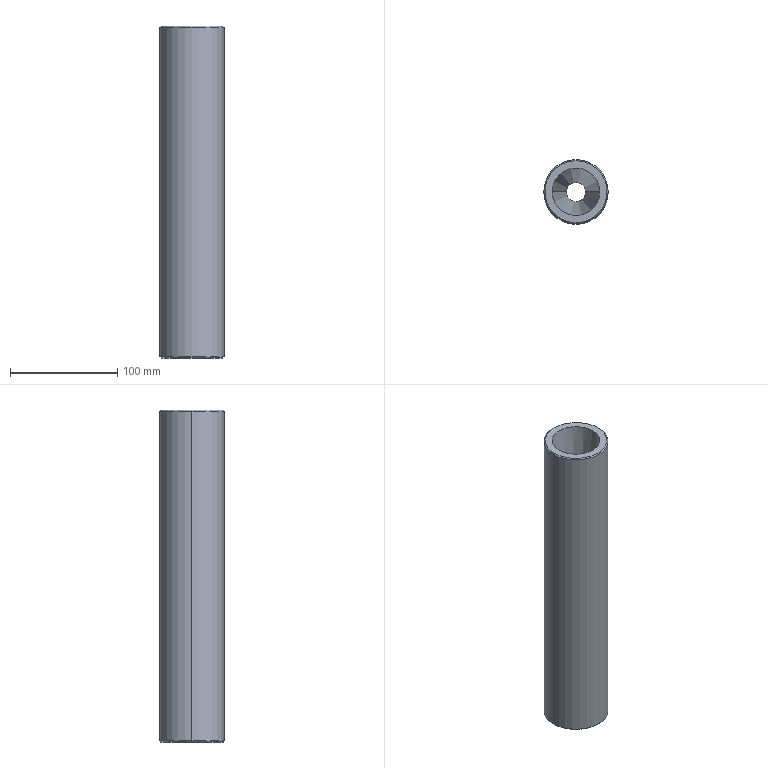Part | STEP file | Tailstock Sleeve | 1 solid | 17 faces | box 60 x 60 x 310 mm | volume 687459 mm3 | cone 8 | cylinder 6 | plane 3 | commonest cylinder face diameters 18 x2 33.5 x2 60 x2
STEP:
#1=CARTESIAN_POINT('',(0.,30.,-154.));
#2=VERTEX_POINT('',#1);
#3=CARTESIAN_POINT('',(-30.,0.,-154.));
#4=VERTEX_POINT('',#3);
#5=CARTESIAN_POINT('',(0.,0.,-154.));
#6=DIRECTION('',(0.,0.,1.));
#7=DIRECTION('',(1.,0.,0.));
#8=AXIS2_PLACEMENT_3D('',#5,#6,#7);
#9=CIRCLE('',#8,30.);
#10=EDGE_CURVE('',#2,#4,#9,.T.);
#11=ORIENTED_EDGE('',*,*,#10,.T.);
#12=CARTESIAN_POINT('',(-30.,0.,154.));
#13=VERTEX_POINT('',#12);
#14=CARTESIAN_POINT('',(-30.,0.,0.));
#15=DIRECTION('',(0.,0.,1.));
#16=VECTOR('',#15,1000.);
#17=LINE('',#14,#16);
#18=EDGE_CURVE('',#4,#13,#17,.T.);
#19=ORIENTED_EDGE('',*,*,#18,.T.);
#20=CARTESIAN_POINT('',(0.,30.,154.));
#21=VERTEX_POINT('',#20);
#22=CARTESIAN_POINT('',(0.,0.,154.));
#23=DIRECTION('',(0.,0.,-1.));
#24=DIRECTION('',(1.,0.,0.));
#25=AXIS2_PLACEMENT_3D('',#22,#23,#24);
#26=CIRCLE('',#25,30.);
#27=EDGE_CURVE('',#13,#21,#26,.T.);
#28=ORIENTED_EDGE('',*,*,#27,.T.);
#29=CARTESIAN_POINT('',(30.,0.,154.));
#30=VERTEX_POINT('',#29);
#31=CARTESIAN_POINT('',(0.,0.,154.));
#32=DIRECTION('',(0.,0.,-1.));
#33=DIRECTION('',(1.,0.,0.));
#34=AXIS2_PLACEMENT_3D('',#31,#32,#33);
#35=CIRCLE('',#34,30.);
#36=EDGE_CURVE('',#21,#30,#35,.T.);
#37=ORIENTED_EDGE('',*,*,#36,.T.);
#38=CARTESIAN_POINT('',(30.,0.,-154.));
#39=VERTEX_POINT('',#38);
#40=CARTESIAN_POINT('',(30.,0.,0.));
#41=DIRECTION('',(0.,0.,1.));
#42=VECTOR('',#41,1000.);
#43=LINE('',#40,#42);
#44=EDGE_CURVE('',#39,#30,#43,.T.);
#45=ORIENTED_EDGE('',*,*,#44,.F.);
#46=CARTESIAN_POINT('',(0.,0.,-154.));
#47=DIRECTION('',(0.,0.,1.));
#48=DIRECTION('',(1.,0.,0.));
#49=AXIS2_PLACEMENT_3D('',#46,#47,#48);
#50=CIRCLE('',#49,30.);
#51=EDGE_CURVE('',#39,#2,#50,.T.);
#52=ORIENTED_EDGE('',*,*,#51,.T.);
#53=EDGE_LOOP('',(#11,#19,#28,#37,#45,#52));
#54=FACE_OUTER_BOUND('',#53,.T.);
#55=CARTESIAN_POINT('',(0.,0.,0.));
#56=DIRECTION('',(0.,0.,1.));
#57=DIRECTION('',(1.,0.,0.));
#58=AXIS2_PLACEMENT_3D('',#55,#56,#57);
#59=CYLINDRICAL_SURFACE('',#58,30.);
#60=ADVANCED_FACE('',(#54),#59,.T.);
#61=CARTESIAN_POINT('',(0.,29.,155.));
#62=VERTEX_POINT('',#61);
#63=CARTESIAN_POINT('',(0.,-29.,155.));
#64=VERTEX_POINT('',#63);
#65=CARTESIAN_POINT('',(0.,0.,155.));
#66=DIRECTION('',(0.,0.,-1.));
#67=DIRECTION('',(0.,1.,0.));
#68=AXIS2_PLACEMENT_3D('',#65,#66,#67);
#69=CIRCLE('',#68,29.);
#70=EDGE_CURVE('',#62,#64,#69,.T.);
#71=ORIENTED_EDGE('',*,*,#70,.T.);
#72=CARTESIAN_POINT('',(0.,-30.,154.));
#73=VERTEX_POINT('',#72);
#74=CARTESIAN_POINT('',(0.,-30.,154.));
#75=DIRECTION('',(0.,-0.7071,-0.7071));
#76=VECTOR('',#75,1000.);
#77=LINE('',#74,#76);
#78=EDGE_CURVE('',#64,#73,#77,.T.);
#79=ORIENTED_EDGE('',*,*,#78,.T.);
#80=CARTESIAN_POINT('',(0.,0.,154.));
#81=DIRECTION('',(0.,0.,-1.));
#82=DIRECTION('',(1.,0.,0.));
#83=AXIS2_PLACEMENT_3D('',#80,#81,#82);
#84=CIRCLE('',#83,30.);
#85=EDGE_CURVE('',#30,#73,#84,.T.);
#86=ORIENTED_EDGE('',*,*,#85,.F.);
#87=ORIENTED_EDGE('',*,*,#36,.F.);
#88=CARTESIAN_POINT('',(0.,30.,154.));
#89=DIRECTION('',(0.,0.7071,-0.7071));
#90=VECTOR('',#89,1000.);
#91=LINE('',#88,#90);
#92=EDGE_CURVE('',#62,#21,#91,.T.);
#93=ORIENTED_EDGE('',*,*,#92,.F.);
#94=EDGE_LOOP('',(#71,#79,#86,#87,#93));
#95=FACE_OUTER_BOUND('',#94,.T.);
#96=CARTESIAN_POINT('',(0.,0.,154.));
#97=DIRECTION('',(0.,0.,-1.));
#98=DIRECTION('',(0.,1.,0.));
#99=AXIS2_PLACEMENT_3D('',#96,#97,#98);
#100=CONICAL_SURFACE('',#99,30.,0.7854);
#101=ADVANCED_FACE('',(#95),#100,.T.);
#102=CARTESIAN_POINT('',(0.,-29.,-155.));
#103=VERTEX_POINT('',#102);
#104=CARTESIAN_POINT('',(0.,29.,-155.));
#105=VERTEX_POINT('',#104);
#106=CARTESIAN_POINT('',(0.,0.,-155.));
#107=DIRECTION('',(0.,0.,1.));
#108=DIRECTION('',(0.,-1.,0.));
#109=AXIS2_PLACEMENT_3D('',#106,#107,#108);
#110=CIRCLE('',#109,29.);
#111=EDGE_CURVE('',#103,#105,#110,.T.);
#112=ORIENTED_EDGE('',*,*,#111,.T.);
#113=CARTESIAN_POINT('',(0.,30.,-154.));
#114=DIRECTION('',(0.,0.7071,0.7071));
#115=VECTOR('',#114,1000.);
#116=LINE('',#113,#115);
#117=EDGE_CURVE('',#105,#2,#116,.T.);
#118=ORIENTED_EDGE('',*,*,#117,.T.);
#119=ORIENTED_EDGE('',*,*,#51,.F.);
#120=CARTESIAN_POINT('',(0.,-30.,-154.));
#121=VERTEX_POINT('',#120);
#122=CARTESIAN_POINT('',(0.,0.,-154.));
#123=DIRECTION('',(0.,0.,1.));
#124=DIRECTION('',(1.,0.,0.));
#125=AXIS2_PLACEMENT_3D('',#122,#123,#124);
#126=CIRCLE('',#125,30.);
#127=EDGE_CURVE('',#121,#39,#126,.T.);
#128=ORIENTED_EDGE('',*,*,#127,.F.);
#129=CARTESIAN_POINT('',(0.,-30.,-154.));
#130=DIRECTION('',(0.,-0.7071,0.7071));
#131=VECTOR('',#130,1000.);
#132=LINE('',#129,#131);
#133=EDGE_CURVE('',#103,#121,#132,.T.);
#134=ORIENTED_EDGE('',*,*,#133,.F.);
#135=EDGE_LOOP('',(#112,#118,#119,#128,#134));
#136=FACE_OUTER_BOUND('',#135,.T.);
#137=CARTESIAN_POINT('',(0.,0.,-154.));
#138=DIRECTION('',(0.,0.,1.));
#139=DIRECTION('',(0.,-1.,0.));
#140=AXIS2_PLACEMENT_3D('',#137,#138,#139);
#141=CONICAL_SURFACE('',#140,30.,0.7854);
#142=ADVANCED_FACE('',(#136),#141,.T.);
#143=CARTESIAN_POINT('',(-9.,0.,13.595));
#144=VERTEX_POINT('',#143);
#145=CARTESIAN_POINT('',(9.,0.,13.595));
#146=VERTEX_POINT('',#145);
#147=CARTESIAN_POINT('',(0.,0.,13.595));
#148=DIRECTION('',(0.,0.,1.));
#149=DIRECTION('',(1.,0.,0.));
#150=AXIS2_PLACEMENT_3D('',#147,#148,#149);
#151=CIRCLE('',#150,9.);
#152=EDGE_CURVE('',#144,#146,#151,.T.);
#153=ORIENTED_EDGE('',*,*,#152,.F.);
#154=CARTESIAN_POINT('',(-22.2,0.,155.));
#155=VERTEX_POINT('',#154);
#156=CARTESIAN_POINT('',(-22.2,0.,155.));
#157=DIRECTION('',(-0.09294,0.,0.9957));
#158=VECTOR('',#157,1000.);
#159=LINE('',#156,#158);
#160=EDGE_CURVE('',#144,#155,#159,.T.);
#161=ORIENTED_EDGE('',*,*,#160,.T.);
#162=CARTESIAN_POINT('',(22.2,0.,155.));
#163=VERTEX_POINT('',#162);
#164=CARTESIAN_POINT('',(0.,0.,155.));
#165=DIRECTION('',(0.,0.,1.));
#166=DIRECTION('',(1.,0.,0.));
#167=AXIS2_PLACEMENT_3D('',#164,#165,#166);
#168=CIRCLE('',#167,22.2);
#169=EDGE_CURVE('',#155,#163,#168,.T.);
#170=ORIENTED_EDGE('',*,*,#169,.T.);
#171=CARTESIAN_POINT('',(22.2,0.,155.));
#172=DIRECTION('',(0.09294,0.,0.9957));
#173=VECTOR('',#172,1000.);
#174=LINE('',#171,#173);
#175=EDGE_CURVE('',#146,#163,#174,.T.);
#176=ORIENTED_EDGE('',*,*,#175,.F.);
#177=EDGE_LOOP('',(#153,#161,#170,#176));
#178=FACE_OUTER_BOUND('',#177,.T.);
#179=CARTESIAN_POINT('',(0.,0.,155.));
#180=DIRECTION('',(0.,0.,1.));
#181=DIRECTION('',(1.,0.,0.));
#182=AXIS2_PLACEMENT_3D('',#179,#180,#181);
#183=CONICAL_SURFACE('',#182,22.2,0.09308);
#184=ADVANCED_FACE('',(#178),#183,.F.);
#185=CARTESIAN_POINT('',(16.75,0.,-154.));
#186=VERTEX_POINT('',#185);
#187=CARTESIAN_POINT('',(-16.75,0.,-154.));
#188=VERTEX_POINT('',#187);
#189=CARTESIAN_POINT('',(0.,0.,-154.));
#190=DIRECTION('',(0.,0.,-1.));
#191=DIRECTION('',(-1.,0.,0.));
#192=AXIS2_PLACEMENT_3D('',#189,#190,#191);
#193=CIRCLE('',#192,16.75);
#194=EDGE_CURVE('',#186,#188,#193,.T.);
#195=ORIENTED_EDGE('',*,*,#194,.F.);
#196=CARTESIAN_POINT('',(17.75,0.,-155.));
#197=VERTEX_POINT('',#196);
#198=CARTESIAN_POINT('',(17.75,0.,-155.));
#199=DIRECTION('',(0.7071,0.,-0.7071));
#200=VECTOR('',#199,1000.);
#201=LINE('',#198,#200);
#202=EDGE_CURVE('',#186,#197,#201,.T.);
#203=ORIENTED_EDGE('',*,*,#202,.T.);
#204=CARTESIAN_POINT('',(-17.75,0.,-155.));
#205=VERTEX_POINT('',#204);
#206=CARTESIAN_POINT('',(0.,0.,-155.));
#207=DIRECTION('',(0.,0.,-1.));
#208=DIRECTION('',(-1.,0.,0.));
#209=AXIS2_PLACEMENT_3D('',#206,#207,#208);
#210=CIRCLE('',#209,17.75);
#211=EDGE_CURVE('',#197,#205,#210,.T.);
#212=ORIENTED_EDGE('',*,*,#211,.T.);
#213=CARTESIAN_POINT('',(-17.75,0.,-155.));
#214=DIRECTION('',(-0.7071,0.,-0.7071));
#215=VECTOR('',#214,1000.);
#216=LINE('',#213,#215);
#217=EDGE_CURVE('',#188,#205,#216,.T.);
#218=ORIENTED_EDGE('',*,*,#217,.F.);
#219=EDGE_LOOP('',(#195,#203,#212,#218));
#220=FACE_OUTER_BOUND('',#219,.T.);
#221=CARTESIAN_POINT('',(0.,0.,-155.));
#222=DIRECTION('',(0.,0.,-1.));
#223=DIRECTION('',(-1.,0.,0.));
#224=AXIS2_PLACEMENT_3D('',#221,#222,#223);
#225=CONICAL_SURFACE('',#224,17.75,0.7854);
#226=ADVANCED_FACE('',(#220),#225,.F.);
#227=CARTESIAN_POINT('',(-9.,0.,-105.));
#228=VERTEX_POINT('',#227);
#229=CARTESIAN_POINT('',(9.,0.,-105.));
#230=VERTEX_POINT('',#229);
#231=CARTESIAN_POINT('',(0.,0.,-105.));
#232=DIRECTION('',(0.,0.,1.));
#233=DIRECTION('',(1.,0.,0.));
#234=AXIS2_PLACEMENT_3D('',#231,#232,#233);
#235=CIRCLE('',#234,9.);
#236=EDGE_CURVE('',#228,#230,#235,.T.);
#237=ORIENTED_EDGE('',*,*,#236,.F.);
#238=CARTESIAN_POINT('',(-9.,0.,0.));
#239=DIRECTION('',(0.,0.,1.));
#240=VECTOR('',#239,1000.);
#241=LINE('',#238,#240);
#242=EDGE_CURVE('',#228,#144,#241,.T.);
#243=ORIENTED_EDGE('',*,*,#242,.T.);
#244=ORIENTED_EDGE('',*,*,#152,.T.);
#245=CARTESIAN_POINT('',(9.,0.,0.));
#246=DIRECTION('',(0.,0.,1.));
#247=VECTOR('',#246,1000.);
#248=LINE('',#245,#247);
#249=EDGE_CURVE('',#230,#146,#248,.T.);
#250=ORIENTED_EDGE('',*,*,#249,.F.);
#251=EDGE_LOOP('',(#237,#243,#244,#250));
#252=FACE_OUTER_BOUND('',#251,.T.);
#253=CARTESIAN_POINT('',(0.,0.,0.));
#254=DIRECTION('',(0.,0.,1.));
#255=DIRECTION('',(1.,0.,0.));
#256=AXIS2_PLACEMENT_3D('',#253,#254,#255);
#257=CYLINDRICAL_SURFACE('',#256,9.);
#258=ADVANCED_FACE('',(#252),#257,.F.);
#259=CARTESIAN_POINT('',(16.75,0.,-105.));
#260=VERTEX_POINT('',#259);
#261=CARTESIAN_POINT('',(-16.75,0.,-105.));
#262=VERTEX_POINT('',#261);
#263=CARTESIAN_POINT('',(0.,0.,-105.));
#264=DIRECTION('',(0.,0.,-1.));
#265=DIRECTION('',(-1.,0.,0.));
#266=AXIS2_PLACEMENT_3D('',#263,#264,#265);
#267=CIRCLE('',#266,16.75);
#268=EDGE_CURVE('',#260,#262,#267,.T.);
#269=ORIENTED_EDGE('',*,*,#268,.F.);
#270=CARTESIAN_POINT('',(16.75,0.,-105.));
#271=DIRECTION('',(0.,0.,-1.));
#272=VECTOR('',#271,1000.);
#273=LINE('',#270,#272);
#274=EDGE_CURVE('',#260,#186,#273,.T.);
#275=ORIENTED_EDGE('',*,*,#274,.T.);
#276=ORIENTED_EDGE('',*,*,#194,.T.);
#277=CARTESIAN_POINT('',(-16.75,0.,-105.));
#278=DIRECTION('',(0.,0.,-1.));
#279=VECTOR('',#278,1000.);
#280=LINE('',#277,#279);
#281=EDGE_CURVE('',#262,#188,#280,.T.);
#282=ORIENTED_EDGE('',*,*,#281,.F.);
#283=EDGE_LOOP('',(#269,#275,#276,#282));
#284=FACE_OUTER_BOUND('',#283,.T.);
#285=CARTESIAN_POINT('',(0.,0.,-105.));
#286=DIRECTION('',(0.,0.,-1.));
#287=DIRECTION('',(-1.,0.,0.));
#288=AXIS2_PLACEMENT_3D('',#285,#286,#287);
#289=CYLINDRICAL_SURFACE('',#288,16.75);
#290=ADVANCED_FACE('',(#284),#289,.F.);
#291=ORIENTED_EDGE('',*,*,#18,.F.);
#292=CARTESIAN_POINT('',(0.,0.,-154.));
#293=DIRECTION('',(0.,0.,1.));
#294=DIRECTION('',(1.,0.,0.));
#295=AXIS2_PLACEMENT_3D('',#292,#293,#294);
#296=CIRCLE('',#295,30.);
#297=EDGE_CURVE('',#4,#121,#296,.T.);
#298=ORIENTED_EDGE('',*,*,#297,.T.);
#299=ORIENTED_EDGE('',*,*,#127,.T.);
#300=ORIENTED_EDGE('',*,*,#44,.T.);
#301=ORIENTED_EDGE('',*,*,#85,.T.);
#302=CARTESIAN_POINT('',(0.,0.,154.));
#303=DIRECTION('',(0.,0.,-1.));
#304=DIRECTION('',(1.,0.,0.));
#305=AXIS2_PLACEMENT_3D('',#302,#303,#304);
#306=CIRCLE('',#305,30.);
#307=EDGE_CURVE('',#73,#13,#306,.T.);
#308=ORIENTED_EDGE('',*,*,#307,.T.);
#309=EDGE_LOOP('',(#291,#298,#299,#300,#301,#308));
#310=FACE_OUTER_BOUND('',#309,.T.);
#311=CARTESIAN_POINT('',(0.,0.,0.));
#312=DIRECTION('',(0.,0.,1.));
#313=DIRECTION('',(1.,0.,0.));
#314=AXIS2_PLACEMENT_3D('',#311,#312,#313);
#315=CYLINDRICAL_SURFACE('',#314,30.);
#316=ADVANCED_FACE('',(#310),#315,.T.);
#317=ORIENTED_EDGE('',*,*,#78,.F.);
#318=CARTESIAN_POINT('',(0.,0.,155.));
#319=DIRECTION('',(0.,0.,-1.));
#320=DIRECTION('',(0.,1.,0.));
#321=AXIS2_PLACEMENT_3D('',#318,#319,#320);
#322=CIRCLE('',#321,29.);
#323=EDGE_CURVE('',#64,#62,#322,.T.);
#324=ORIENTED_EDGE('',*,*,#323,.T.);
#325=ORIENTED_EDGE('',*,*,#92,.T.);
#326=ORIENTED_EDGE('',*,*,#27,.F.);
#327=ORIENTED_EDGE('',*,*,#307,.F.);
#328=EDGE_LOOP('',(#317,#324,#325,#326,#327));
#329=FACE_OUTER_BOUND('',#328,.T.);
#330=CARTESIAN_POINT('',(0.,0.,154.));
#331=DIRECTION('',(0.,0.,-1.));
#332=DIRECTION('',(0.,1.,0.));
#333=AXIS2_PLACEMENT_3D('',#330,#331,#332);
#334=CONICAL_SURFACE('',#333,30.,0.7854);
#335=ADVANCED_FACE('',(#329),#334,.T.);
#336=ORIENTED_EDGE('',*,*,#117,.F.);
#337=CARTESIAN_POINT('',(0.,0.,-155.));
#338=DIRECTION('',(0.,0.,1.));
#339=DIRECTION('',(0.,-1.,0.));
#340=AXIS2_PLACEMENT_3D('',#337,#338,#339);
#341=CIRCLE('',#340,29.);
#342=EDGE_CURVE('',#105,#103,#341,.T.);
#343=ORIENTED_EDGE('',*,*,#342,.T.);
#344=ORIENTED_EDGE('',*,*,#133,.T.);
#345=ORIENTED_EDGE('',*,*,#297,.F.);
#346=ORIENTED_EDGE('',*,*,#10,.F.);
#347=EDGE_LOOP('',(#336,#343,#344,#345,#346));
#348=FACE_OUTER_BOUND('',#347,.T.);
#349=CARTESIAN_POINT('',(0.,0.,-154.));
#350=DIRECTION('',(0.,0.,1.));
#351=DIRECTION('',(0.,-1.,0.));
#352=AXIS2_PLACEMENT_3D('',#349,#350,#351);
#353=CONICAL_SURFACE('',#352,30.,0.7854);
#354=ADVANCED_FACE('',(#348),#353,.T.);
#355=CARTESIAN_POINT('',(0.,0.,155.));
#356=DIRECTION('',(0.,0.,1.));
#357=DIRECTION('',(1.,0.,0.));
#358=AXIS2_PLACEMENT_3D('',#355,#356,#357);
#359=CIRCLE('',#358,22.2);
#360=EDGE_CURVE('',#163,#155,#359,.T.);
#361=ORIENTED_EDGE('',*,*,#360,.F.);
#362=ORIENTED_EDGE('',*,*,#169,.F.);
#363=EDGE_LOOP('',(#361,#362));
#364=FACE_BOUND('',#363,.T.);
#365=ORIENTED_EDGE('',*,*,#70,.F.);
#366=ORIENTED_EDGE('',*,*,#323,.F.);
#367=EDGE_LOOP('',(#365,#366));
#368=FACE_OUTER_BOUND('',#367,.T.);
#369=CARTESIAN_POINT('',(0.,30.,155.));
#370=DIRECTION('',(0.,0.,-1.));
#371=DIRECTION('',(-1.,0.,0.));
#372=AXIS2_PLACEMENT_3D('',#369,#370,#371);
#373=PLANE('',#372);
#374=ADVANCED_FACE('',(#364,#368),#373,.F.);
#375=ORIENTED_EDGE('',*,*,#111,.F.);
#376=ORIENTED_EDGE('',*,*,#342,.F.);
#377=EDGE_LOOP('',(#375,#376));
#378=FACE_OUTER_BOUND('',#377,.T.);
#379=CARTESIAN_POINT('',(0.,0.,-155.));
#380=DIRECTION('',(0.,0.,-1.));
#381=DIRECTION('',(-1.,0.,0.));
#382=AXIS2_PLACEMENT_3D('',#379,#380,#381);
#383=CIRCLE('',#382,17.75);
#384=EDGE_CURVE('',#205,#197,#383,.T.);
#385=ORIENTED_EDGE('',*,*,#384,.F.);
#386=ORIENTED_EDGE('',*,*,#211,.F.);
#387=EDGE_LOOP('',(#385,#386));
#388=FACE_BOUND('',#387,.T.);
#389=CARTESIAN_POINT('',(0.,30.,-155.));
#390=DIRECTION('',(0.,0.,1.));
#391=DIRECTION('',(1.,0.,0.));
#392=AXIS2_PLACEMENT_3D('',#389,#390,#391);
#393=PLANE('',#392);
#394=ADVANCED_FACE('',(#378,#388),#393,.F.);
#395=ORIENTED_EDGE('',*,*,#160,.F.);
#396=CARTESIAN_POINT('',(0.,0.,13.595));
#397=DIRECTION('',(0.,0.,1.));
#398=DIRECTION('',(1.,0.,0.));
#399=AXIS2_PLACEMENT_3D('',#396,#397,#398);
#400=CIRCLE('',#399,9.);
#401=EDGE_CURVE('',#146,#144,#400,.T.);
#402=ORIENTED_EDGE('',*,*,#401,.F.);
#403=ORIENTED_EDGE('',*,*,#175,.T.);
#404=ORIENTED_EDGE('',*,*,#360,.T.);
#405=EDGE_LOOP('',(#395,#402,#403,#404));
#406=FACE_OUTER_BOUND('',#405,.T.);
#407=CARTESIAN_POINT('',(0.,0.,155.));
#408=DIRECTION('',(0.,0.,1.));
#409=DIRECTION('',(1.,0.,0.));
#410=AXIS2_PLACEMENT_3D('',#407,#408,#409);
#411=CONICAL_SURFACE('',#410,22.2,0.09308);
#412=ADVANCED_FACE('',(#406),#411,.F.);
#413=ORIENTED_EDGE('',*,*,#202,.F.);
#414=CARTESIAN_POINT('',(0.,0.,-154.));
#415=DIRECTION('',(0.,0.,-1.));
#416=DIRECTION('',(-1.,0.,0.));
#417=AXIS2_PLACEMENT_3D('',#414,#415,#416);
#418=CIRCLE('',#417,16.75);
#419=EDGE_CURVE('',#188,#186,#418,.T.);
#420=ORIENTED_EDGE('',*,*,#419,.F.);
#421=ORIENTED_EDGE('',*,*,#217,.T.);
#422=ORIENTED_EDGE('',*,*,#384,.T.);
#423=EDGE_LOOP('',(#413,#420,#421,#422));
#424=FACE_OUTER_BOUND('',#423,.T.);
#425=CARTESIAN_POINT('',(0.,0.,-155.));
#426=DIRECTION('',(0.,0.,-1.));
#427=DIRECTION('',(-1.,0.,0.));
#428=AXIS2_PLACEMENT_3D('',#425,#426,#427);
#429=CONICAL_SURFACE('',#428,17.75,0.7854);
#430=ADVANCED_FACE('',(#424),#429,.F.);
#431=ORIENTED_EDGE('',*,*,#242,.F.);
#432=CARTESIAN_POINT('',(0.,0.,-105.));
#433=DIRECTION('',(0.,0.,1.));
#434=DIRECTION('',(1.,0.,0.));
#435=AXIS2_PLACEMENT_3D('',#432,#433,#434);
#436=CIRCLE('',#435,9.);
#437=EDGE_CURVE('',#230,#228,#436,.T.);
#438=ORIENTED_EDGE('',*,*,#437,.F.);
#439=ORIENTED_EDGE('',*,*,#249,.T.);
#440=ORIENTED_EDGE('',*,*,#401,.T.);
#441=EDGE_LOOP('',(#431,#438,#439,#440));
#442=FACE_OUTER_BOUND('',#441,.T.);
#443=CARTESIAN_POINT('',(0.,0.,0.));
#444=DIRECTION('',(0.,0.,1.));
#445=DIRECTION('',(1.,0.,0.));
#446=AXIS2_PLACEMENT_3D('',#443,#444,#445);
#447=CYLINDRICAL_SURFACE('',#446,9.);
#448=ADVANCED_FACE('',(#442),#447,.F.);
#449=ORIENTED_EDGE('',*,*,#274,.F.);
#450=CARTESIAN_POINT('',(0.,0.,-105.));
#451=DIRECTION('',(0.,0.,-1.));
#452=DIRECTION('',(-1.,0.,0.));
#453=AXIS2_PLACEMENT_3D('',#450,#451,#452);
#454=CIRCLE('',#453,16.75);
#455=EDGE_CURVE('',#262,#260,#454,.T.);
#456=ORIENTED_EDGE('',*,*,#455,.F.);
#457=ORIENTED_EDGE('',*,*,#281,.T.);
#458=ORIENTED_EDGE('',*,*,#419,.T.);
#459=EDGE_LOOP('',(#449,#456,#457,#458));
#460=FACE_OUTER_BOUND('',#459,.T.);
#461=CARTESIAN_POINT('',(0.,0.,-105.));
#462=DIRECTION('',(0.,0.,-1.));
#463=DIRECTION('',(-1.,0.,0.));
#464=AXIS2_PLACEMENT_3D('',#461,#462,#463);
#465=CYLINDRICAL_SURFACE('',#464,16.75);
#466=ADVANCED_FACE('',(#460),#465,.F.);
#467=ORIENTED_EDGE('',*,*,#437,.T.);
#468=ORIENTED_EDGE('',*,*,#236,.T.);
#469=EDGE_LOOP('',(#467,#468));
#470=FACE_BOUND('',#469,.T.);
#471=ORIENTED_EDGE('',*,*,#455,.T.);
#472=ORIENTED_EDGE('',*,*,#268,.T.);
#473=EDGE_LOOP('',(#471,#472));
#474=FACE_OUTER_BOUND('',#473,.T.);
#475=CARTESIAN_POINT('',(0.,0.,-105.));
#476=DIRECTION('',(0.,0.,-1.));
#477=DIRECTION('',(-1.,0.,0.));
#478=AXIS2_PLACEMENT_3D('',#475,#476,#477);
#479=PLANE('',#478);
#480=ADVANCED_FACE('',(#470,#474),#479,.T.);
#481=CLOSED_SHELL('',(#60,#101,#142,#184,#226,#258,#290,#316,#335,#354,#374,#394,#412,#430,#448,#466,#480));
#482=MANIFOLD_SOLID_BREP('',#481);
#483=CARTESIAN_POINT('',(0.,0.,0.));
#484=DIRECTION('',(0.,0.,1.));
#485=DIRECTION('',(1.,0.,0.));
#486=AXIS2_PLACEMENT_3D('',#483,#484,#485);
#487=(LENGTH_UNIT()NAMED_UNIT(*)SI_UNIT(.MILLI.,.METRE.));
#488=UNCERTAINTY_MEASURE_WITH_UNIT(LENGTH_MEASURE(0.00001),#487,'','');
#489=(NAMED_UNIT(*)PLANE_ANGLE_UNIT()SI_UNIT($,.RADIAN.));
#490=(NAMED_UNIT(*)SI_UNIT($,.STERADIAN.)SOLID_ANGLE_UNIT());
#491=(GEOMETRIC_REPRESENTATION_CONTEXT(3)GLOBAL_UNCERTAINTY_ASSIGNED_CONTEXT((#488))GLOBAL_UNIT_ASSIGNED_CONTEXT((#487,#489,#490))REPRESENTATION_CONTEXT('',''));
#492=ADVANCED_BREP_SHAPE_REPRESENTATION('',(#482,#486),#491);